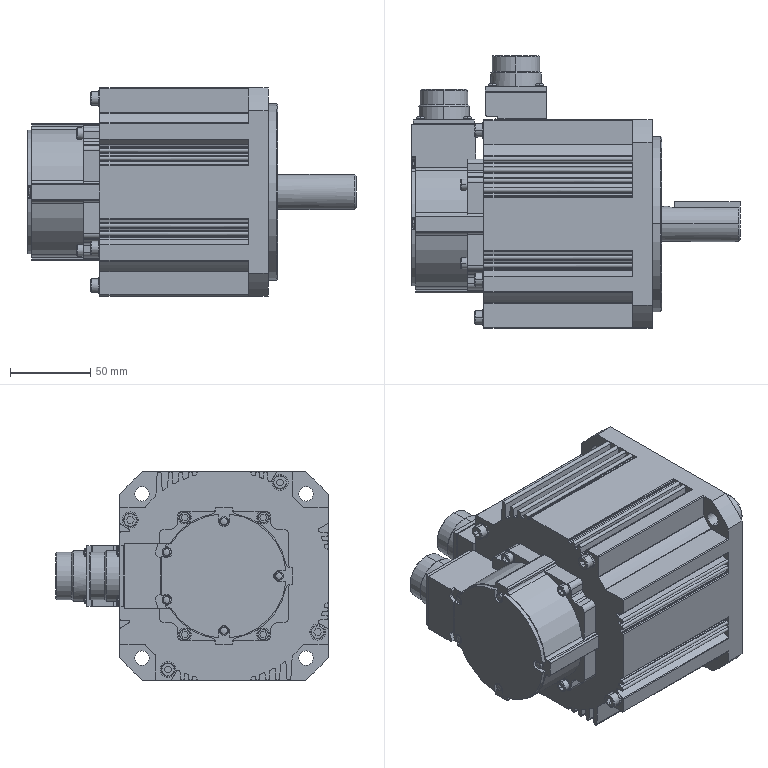Part | SolidWorks | features BaseBody 1 | 1 solid | 667 faces | box 205 x 170 x 130 mm | volume 1936135 mm3 | cylinder 305 | plane 268 | cone 48 | spline 46 | commonest cylinder face diameters 1 x90 2 x30 131 x24 2.5 x22 4 x20 5.6 x10